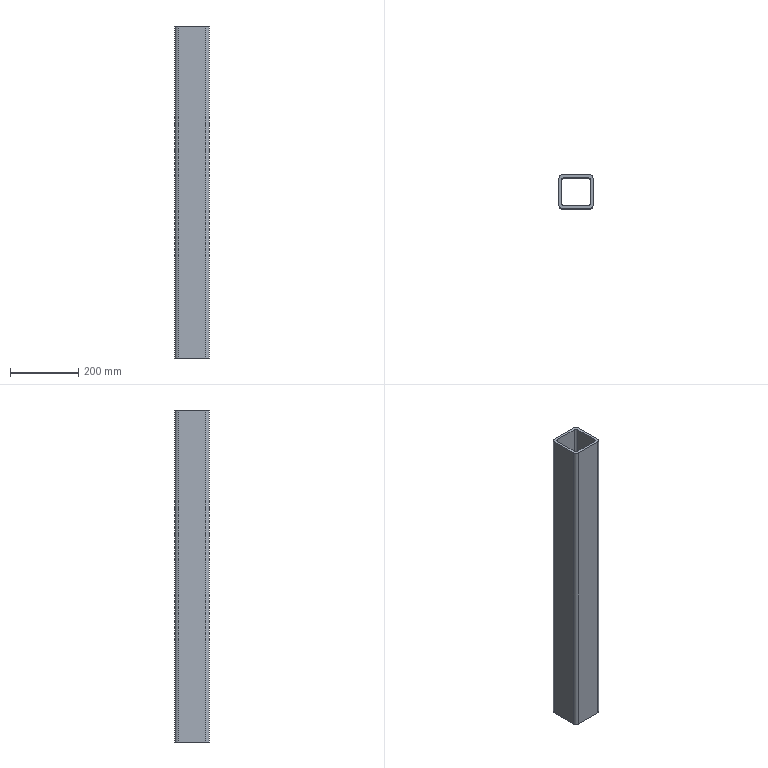Part | SolidWorks | features BaseBody 1 | 1 solid | 18 faces | box 100 x 100 x 976 mm | volume 2843183 mm3 | plane 10 | cylinder 8 | commonest cylinder face diameters 16 x4 20 x4
STEP:
#1=CARTESIAN_POINT('',(90.,-3.65,976.));
#2=VERTEX_POINT('',#1);
#3=CARTESIAN_POINT('',(90.,-3.65,0.));
#4=VERTEX_POINT('',#3);
#5=CARTESIAN_POINT('',(90.,-3.65,976.));
#6=DIRECTION('',(0.,0.,-1.));
#7=VECTOR('',#6,1000.);
#8=LINE('',#5,#7);
#9=EDGE_CURVE('',#2,#4,#8,.T.);
#10=ORIENTED_EDGE('',*,*,#9,.F.);
#11=CARTESIAN_POINT('',(10.,-3.65,976.));
#12=VERTEX_POINT('',#11);
#13=CARTESIAN_POINT('',(10.,-3.65,976.));
#14=DIRECTION('',(1.,0.,0.));
#15=VECTOR('',#14,1000.);
#16=LINE('',#13,#15);
#17=EDGE_CURVE('',#12,#2,#16,.T.);
#18=ORIENTED_EDGE('',*,*,#17,.F.);
#19=CARTESIAN_POINT('',(10.,-3.65,0.));
#20=VERTEX_POINT('',#19);
#21=CARTESIAN_POINT('',(10.,-3.65,976.));
#22=DIRECTION('',(0.,0.,1.));
#23=VECTOR('',#22,1000.);
#24=LINE('',#21,#23);
#25=EDGE_CURVE('',#20,#12,#24,.T.);
#26=ORIENTED_EDGE('',*,*,#25,.F.);
#27=CARTESIAN_POINT('',(10.,-3.65,0.));
#28=DIRECTION('',(-1.,0.,0.));
#29=VECTOR('',#28,1000.);
#30=LINE('',#27,#29);
#31=EDGE_CURVE('',#4,#20,#30,.T.);
#32=ORIENTED_EDGE('',*,*,#31,.F.);
#33=EDGE_LOOP('',(#10,#18,#26,#32));
#34=FACE_OUTER_BOUND('',#33,.T.);
#35=CARTESIAN_POINT('',(10.,-3.65,976.));
#36=DIRECTION('',(0.,1.,0.));
#37=DIRECTION('',(-1.,0.,0.));
#38=AXIS2_PLACEMENT_3D('',#35,#36,#37);
#39=PLANE('',#38);
#40=ADVANCED_FACE('',(#34),#39,.F.);
#41=CARTESIAN_POINT('',(84.,4.35,0.));
#42=VERTEX_POINT('',#41);
#43=CARTESIAN_POINT('',(16.,4.35,0.));
#44=VERTEX_POINT('',#43);
#45=CARTESIAN_POINT('',(10.,4.35,0.));
#46=DIRECTION('',(-1.,0.,0.));
#47=VECTOR('',#46,1000.);
#48=LINE('',#45,#47);
#49=EDGE_CURVE('',#42,#44,#48,.T.);
#50=ORIENTED_EDGE('',*,*,#49,.F.);
#51=CARTESIAN_POINT('',(92.,12.35,0.));
#52=VERTEX_POINT('',#51);
#53=CARTESIAN_POINT('',(84.,12.35,0.));
#54=DIRECTION('',(0.,0.,-1.));
#55=DIRECTION('',(-1.,0.,0.));
#56=AXIS2_PLACEMENT_3D('',#53,#54,#55);
#57=CIRCLE('',#56,8.);
#58=EDGE_CURVE('',#52,#42,#57,.T.);
#59=ORIENTED_EDGE('',*,*,#58,.F.);
#60=CARTESIAN_POINT('',(92.,80.35,0.));
#61=VERTEX_POINT('',#60);
#62=CARTESIAN_POINT('',(92.,6.35,0.));
#63=DIRECTION('',(0.,-1.,0.));
#64=VECTOR('',#63,1000.);
#65=LINE('',#62,#64);
#66=EDGE_CURVE('',#61,#52,#65,.T.);
#67=ORIENTED_EDGE('',*,*,#66,.F.);
#68=CARTESIAN_POINT('',(84.,88.35,0.));
#69=VERTEX_POINT('',#68);
#70=CARTESIAN_POINT('',(84.,80.35,0.));
#71=DIRECTION('',(0.,0.,-1.));
#72=DIRECTION('',(-1.,0.,0.));
#73=AXIS2_PLACEMENT_3D('',#70,#71,#72);
#74=CIRCLE('',#73,8.);
#75=EDGE_CURVE('',#69,#61,#74,.T.);
#76=ORIENTED_EDGE('',*,*,#75,.F.);
#77=CARTESIAN_POINT('',(16.,88.35,0.));
#78=VERTEX_POINT('',#77);
#79=CARTESIAN_POINT('',(10.,88.35,0.));
#80=DIRECTION('',(1.,0.,0.));
#81=VECTOR('',#80,1000.);
#82=LINE('',#79,#81);
#83=EDGE_CURVE('',#78,#69,#82,.T.);
#84=ORIENTED_EDGE('',*,*,#83,.F.);
#85=CARTESIAN_POINT('',(8.,80.35,0.));
#86=VERTEX_POINT('',#85);
#87=CARTESIAN_POINT('',(16.,80.35,0.));
#88=DIRECTION('',(0.,0.,-1.));
#89=DIRECTION('',(-1.,0.,0.));
#90=AXIS2_PLACEMENT_3D('',#87,#88,#89);
#91=CIRCLE('',#90,8.);
#92=EDGE_CURVE('',#86,#78,#91,.T.);
#93=ORIENTED_EDGE('',*,*,#92,.F.);
#94=CARTESIAN_POINT('',(8.,12.35,0.));
#95=VERTEX_POINT('',#94);
#96=CARTESIAN_POINT('',(8.,6.35,0.));
#97=DIRECTION('',(0.,1.,0.));
#98=VECTOR('',#97,1000.);
#99=LINE('',#96,#98);
#100=EDGE_CURVE('',#95,#86,#99,.T.);
#101=ORIENTED_EDGE('',*,*,#100,.F.);
#102=CARTESIAN_POINT('',(16.,12.35,0.));
#103=DIRECTION('',(0.,0.,-1.));
#104=DIRECTION('',(-1.,0.,0.));
#105=AXIS2_PLACEMENT_3D('',#102,#103,#104);
#106=CIRCLE('',#105,8.);
#107=EDGE_CURVE('',#44,#95,#106,.T.);
#108=ORIENTED_EDGE('',*,*,#107,.F.);
#109=EDGE_LOOP('',(#50,#59,#67,#76,#84,#93,#101,#108));
#110=FACE_BOUND('',#109,.T.);
#111=CARTESIAN_POINT('',(0.,86.35,0.));
#112=VERTEX_POINT('',#111);
#113=CARTESIAN_POINT('',(0.,6.35,0.));
#114=VERTEX_POINT('',#113);
#115=CARTESIAN_POINT('',(0.,6.35,0.));
#116=DIRECTION('',(0.,-1.,0.));
#117=VECTOR('',#116,1000.);
#118=LINE('',#115,#117);
#119=EDGE_CURVE('',#112,#114,#118,.T.);
#120=ORIENTED_EDGE('',*,*,#119,.F.);
#121=CARTESIAN_POINT('',(10.,96.35,0.));
#122=VERTEX_POINT('',#121);
#123=CARTESIAN_POINT('',(10.,86.35,0.));
#124=DIRECTION('',(0.,0.,1.));
#125=DIRECTION('',(-1.,0.,0.));
#126=AXIS2_PLACEMENT_3D('',#123,#124,#125);
#127=CIRCLE('',#126,10.);
#128=EDGE_CURVE('',#122,#112,#127,.T.);
#129=ORIENTED_EDGE('',*,*,#128,.F.);
#130=CARTESIAN_POINT('',(90.,96.35,0.));
#131=VERTEX_POINT('',#130);
#132=CARTESIAN_POINT('',(10.,96.35,0.));
#133=DIRECTION('',(-1.,0.,0.));
#134=VECTOR('',#133,1000.);
#135=LINE('',#132,#134);
#136=EDGE_CURVE('',#131,#122,#135,.T.);
#137=ORIENTED_EDGE('',*,*,#136,.F.);
#138=CARTESIAN_POINT('',(100.,86.35,0.));
#139=VERTEX_POINT('',#138);
#140=CARTESIAN_POINT('',(90.,86.35,0.));
#141=DIRECTION('',(0.,0.,1.));
#142=DIRECTION('',(-1.,0.,0.));
#143=AXIS2_PLACEMENT_3D('',#140,#141,#142);
#144=CIRCLE('',#143,10.);
#145=EDGE_CURVE('',#139,#131,#144,.T.);
#146=ORIENTED_EDGE('',*,*,#145,.F.);
#147=CARTESIAN_POINT('',(100.,6.35,0.));
#148=VERTEX_POINT('',#147);
#149=CARTESIAN_POINT('',(100.,6.35,0.));
#150=DIRECTION('',(0.,1.,0.));
#151=VECTOR('',#150,1000.);
#152=LINE('',#149,#151);
#153=EDGE_CURVE('',#148,#139,#152,.T.);
#154=ORIENTED_EDGE('',*,*,#153,.F.);
#155=CARTESIAN_POINT('',(90.,6.35,0.));
#156=DIRECTION('',(0.,0.,1.));
#157=DIRECTION('',(-1.,0.,0.));
#158=AXIS2_PLACEMENT_3D('',#155,#156,#157);
#159=CIRCLE('',#158,10.);
#160=EDGE_CURVE('',#4,#148,#159,.T.);
#161=ORIENTED_EDGE('',*,*,#160,.F.);
#162=ORIENTED_EDGE('',*,*,#31,.T.);
#163=CARTESIAN_POINT('',(10.,6.35,0.));
#164=DIRECTION('',(0.,0.,1.));
#165=DIRECTION('',(-1.,0.,0.));
#166=AXIS2_PLACEMENT_3D('',#163,#164,#165);
#167=CIRCLE('',#166,10.);
#168=EDGE_CURVE('',#114,#20,#167,.T.);
#169=ORIENTED_EDGE('',*,*,#168,.F.);
#170=EDGE_LOOP('',(#120,#129,#137,#146,#154,#161,#162,#169));
#171=FACE_OUTER_BOUND('',#170,.T.);
#172=CARTESIAN_POINT('',(10.,6.35,0.));
#173=DIRECTION('',(0.,0.,1.));
#174=DIRECTION('',(1.,0.,0.));
#175=AXIS2_PLACEMENT_3D('',#172,#173,#174);
#176=PLANE('',#175);
#177=ADVANCED_FACE('',(#110,#171),#176,.F.);
#178=CARTESIAN_POINT('',(100.,6.35,976.));
#179=VERTEX_POINT('',#178);
#180=CARTESIAN_POINT('',(90.,6.35,976.));
#181=DIRECTION('',(0.,0.,-1.));
#182=DIRECTION('',(-1.,0.,0.));
#183=AXIS2_PLACEMENT_3D('',#180,#181,#182);
#184=CIRCLE('',#183,10.);
#185=EDGE_CURVE('',#179,#2,#184,.T.);
#186=ORIENTED_EDGE('',*,*,#185,.T.);
#187=ORIENTED_EDGE('',*,*,#9,.T.);
#188=ORIENTED_EDGE('',*,*,#160,.T.);
#189=CARTESIAN_POINT('',(100.,6.35,976.));
#190=DIRECTION('',(0.,0.,1.));
#191=VECTOR('',#190,1000.);
#192=LINE('',#189,#191);
#193=EDGE_CURVE('',#148,#179,#192,.T.);
#194=ORIENTED_EDGE('',*,*,#193,.T.);
#195=EDGE_LOOP('',(#186,#187,#188,#194));
#196=FACE_OUTER_BOUND('',#195,.T.);
#197=CARTESIAN_POINT('',(90.,6.35,976.));
#198=DIRECTION('',(0.,0.,-1.));
#199=DIRECTION('',(-1.,0.,0.));
#200=AXIS2_PLACEMENT_3D('',#197,#198,#199);
#201=CYLINDRICAL_SURFACE('',#200,10.);
#202=ADVANCED_FACE('',(#196),#201,.T.);
#203=CARTESIAN_POINT('',(92.,80.35,976.));
#204=VERTEX_POINT('',#203);
#205=CARTESIAN_POINT('',(92.,12.35,976.));
#206=VERTEX_POINT('',#205);
#207=CARTESIAN_POINT('',(92.,6.35,976.));
#208=DIRECTION('',(0.,-1.,0.));
#209=VECTOR('',#208,1000.);
#210=LINE('',#207,#209);
#211=EDGE_CURVE('',#204,#206,#210,.T.);
#212=ORIENTED_EDGE('',*,*,#211,.T.);
#213=CARTESIAN_POINT('',(84.,4.35,976.));
#214=VERTEX_POINT('',#213);
#215=CARTESIAN_POINT('',(84.,12.35,976.));
#216=DIRECTION('',(0.,0.,-1.));
#217=DIRECTION('',(-1.,0.,0.));
#218=AXIS2_PLACEMENT_3D('',#215,#216,#217);
#219=CIRCLE('',#218,8.);
#220=EDGE_CURVE('',#206,#214,#219,.T.);
#221=ORIENTED_EDGE('',*,*,#220,.T.);
#222=CARTESIAN_POINT('',(16.,4.35,976.));
#223=VERTEX_POINT('',#222);
#224=CARTESIAN_POINT('',(10.,4.35,976.));
#225=DIRECTION('',(-1.,0.,0.));
#226=VECTOR('',#225,1000.);
#227=LINE('',#224,#226);
#228=EDGE_CURVE('',#214,#223,#227,.T.);
#229=ORIENTED_EDGE('',*,*,#228,.T.);
#230=CARTESIAN_POINT('',(8.,12.35,976.));
#231=VERTEX_POINT('',#230);
#232=CARTESIAN_POINT('',(16.,12.35,976.));
#233=DIRECTION('',(0.,0.,-1.));
#234=DIRECTION('',(-1.,0.,0.));
#235=AXIS2_PLACEMENT_3D('',#232,#233,#234);
#236=CIRCLE('',#235,8.);
#237=EDGE_CURVE('',#223,#231,#236,.T.);
#238=ORIENTED_EDGE('',*,*,#237,.T.);
#239=CARTESIAN_POINT('',(8.,80.35,976.));
#240=VERTEX_POINT('',#239);
#241=CARTESIAN_POINT('',(8.,6.35,976.));
#242=DIRECTION('',(0.,1.,0.));
#243=VECTOR('',#242,1000.);
#244=LINE('',#241,#243);
#245=EDGE_CURVE('',#231,#240,#244,.T.);
#246=ORIENTED_EDGE('',*,*,#245,.T.);
#247=CARTESIAN_POINT('',(16.,88.35,976.));
#248=VERTEX_POINT('',#247);
#249=CARTESIAN_POINT('',(16.,80.35,976.));
#250=DIRECTION('',(0.,0.,-1.));
#251=DIRECTION('',(-1.,0.,0.));
#252=AXIS2_PLACEMENT_3D('',#249,#250,#251);
#253=CIRCLE('',#252,8.);
#254=EDGE_CURVE('',#240,#248,#253,.T.);
#255=ORIENTED_EDGE('',*,*,#254,.T.);
#256=CARTESIAN_POINT('',(84.,88.35,976.));
#257=VERTEX_POINT('',#256);
#258=CARTESIAN_POINT('',(10.,88.35,976.));
#259=DIRECTION('',(1.,0.,0.));
#260=VECTOR('',#259,1000.);
#261=LINE('',#258,#260);
#262=EDGE_CURVE('',#248,#257,#261,.T.);
#263=ORIENTED_EDGE('',*,*,#262,.T.);
#264=CARTESIAN_POINT('',(84.,80.35,976.));
#265=DIRECTION('',(0.,0.,-1.));
#266=DIRECTION('',(-1.,0.,0.));
#267=AXIS2_PLACEMENT_3D('',#264,#265,#266);
#268=CIRCLE('',#267,8.);
#269=EDGE_CURVE('',#257,#204,#268,.T.);
#270=ORIENTED_EDGE('',*,*,#269,.T.);
#271=EDGE_LOOP('',(#212,#221,#229,#238,#246,#255,#263,#270));
#272=FACE_BOUND('',#271,.T.);
#273=CARTESIAN_POINT('',(10.,96.35,976.));
#274=VERTEX_POINT('',#273);
#275=CARTESIAN_POINT('',(0.,86.35,976.));
#276=VERTEX_POINT('',#275);
#277=CARTESIAN_POINT('',(10.,86.35,976.));
#278=DIRECTION('',(0.,0.,1.));
#279=DIRECTION('',(-1.,0.,0.));
#280=AXIS2_PLACEMENT_3D('',#277,#278,#279);
#281=CIRCLE('',#280,10.);
#282=EDGE_CURVE('',#274,#276,#281,.T.);
#283=ORIENTED_EDGE('',*,*,#282,.T.);
#284=CARTESIAN_POINT('',(0.,6.35,976.));
#285=VERTEX_POINT('',#284);
#286=CARTESIAN_POINT('',(0.,6.35,976.));
#287=DIRECTION('',(0.,-1.,0.));
#288=VECTOR('',#287,1000.);
#289=LINE('',#286,#288);
#290=EDGE_CURVE('',#276,#285,#289,.T.);
#291=ORIENTED_EDGE('',*,*,#290,.T.);
#292=CARTESIAN_POINT('',(10.,6.35,976.));
#293=DIRECTION('',(0.,0.,1.));
#294=DIRECTION('',(-1.,0.,0.));
#295=AXIS2_PLACEMENT_3D('',#292,#293,#294);
#296=CIRCLE('',#295,10.);
#297=EDGE_CURVE('',#285,#12,#296,.T.);
#298=ORIENTED_EDGE('',*,*,#297,.T.);
#299=ORIENTED_EDGE('',*,*,#17,.T.);
#300=ORIENTED_EDGE('',*,*,#185,.F.);
#301=CARTESIAN_POINT('',(100.,86.35,976.));
#302=VERTEX_POINT('',#301);
#303=CARTESIAN_POINT('',(100.,6.35,976.));
#304=DIRECTION('',(0.,1.,0.));
#305=VECTOR('',#304,1000.);
#306=LINE('',#303,#305);
#307=EDGE_CURVE('',#179,#302,#306,.T.);
#308=ORIENTED_EDGE('',*,*,#307,.T.);
#309=CARTESIAN_POINT('',(90.,96.35,976.));
#310=VERTEX_POINT('',#309);
#311=CARTESIAN_POINT('',(90.,86.35,976.));
#312=DIRECTION('',(0.,0.,1.));
#313=DIRECTION('',(-1.,0.,0.));
#314=AXIS2_PLACEMENT_3D('',#311,#312,#313);
#315=CIRCLE('',#314,10.);
#316=EDGE_CURVE('',#302,#310,#315,.T.);
#317=ORIENTED_EDGE('',*,*,#316,.T.);
#318=CARTESIAN_POINT('',(10.,96.35,976.));
#319=DIRECTION('',(-1.,0.,0.));
#320=VECTOR('',#319,1000.);
#321=LINE('',#318,#320);
#322=EDGE_CURVE('',#310,#274,#321,.T.);
#323=ORIENTED_EDGE('',*,*,#322,.T.);
#324=EDGE_LOOP('',(#283,#291,#298,#299,#300,#308,#317,#323));
#325=FACE_OUTER_BOUND('',#324,.T.);
#326=CARTESIAN_POINT('',(10.,6.35,976.));
#327=DIRECTION('',(0.,0.,1.));
#328=DIRECTION('',(1.,0.,0.));
#329=AXIS2_PLACEMENT_3D('',#326,#327,#328);
#330=PLANE('',#329);
#331=ADVANCED_FACE('',(#272,#325),#330,.T.);
#332=ORIENTED_EDGE('',*,*,#297,.F.);
#333=CARTESIAN_POINT('',(0.,6.35,976.));
#334=DIRECTION('',(0.,0.,-1.));
#335=VECTOR('',#334,1000.);
#336=LINE('',#333,#335);
#337=EDGE_CURVE('',#285,#114,#336,.T.);
#338=ORIENTED_EDGE('',*,*,#337,.T.);
#339=ORIENTED_EDGE('',*,*,#168,.T.);
#340=ORIENTED_EDGE('',*,*,#25,.T.);
#341=EDGE_LOOP('',(#332,#338,#339,#340));
#342=FACE_OUTER_BOUND('',#341,.T.);
#343=CARTESIAN_POINT('',(10.,6.35,976.));
#344=DIRECTION('',(0.,0.,-1.));
#345=DIRECTION('',(-1.,0.,0.));
#346=AXIS2_PLACEMENT_3D('',#343,#344,#345);
#347=CYLINDRICAL_SURFACE('',#346,10.);
#348=ADVANCED_FACE('',(#342),#347,.T.);
#349=CARTESIAN_POINT('',(8.,12.35,976.));
#350=DIRECTION('',(0.,0.,-1.));
#351=VECTOR('',#350,1000.);
#352=LINE('',#349,#351);
#353=EDGE_CURVE('',#231,#95,#352,.T.);
#354=ORIENTED_EDGE('',*,*,#353,.F.);
#355=ORIENTED_EDGE('',*,*,#237,.F.);
#356=CARTESIAN_POINT('',(16.,4.35,976.));
#357=DIRECTION('',(0.,0.,1.));
#358=VECTOR('',#357,1000.);
#359=LINE('',#356,#358);
#360=EDGE_CURVE('',#44,#223,#359,.T.);
#361=ORIENTED_EDGE('',*,*,#360,.F.);
#362=ORIENTED_EDGE('',*,*,#107,.T.);
#363=EDGE_LOOP('',(#354,#355,#361,#362));
#364=FACE_OUTER_BOUND('',#363,.T.);
#365=CARTESIAN_POINT('',(16.,12.35,976.));
#366=DIRECTION('',(0.,0.,-1.));
#367=DIRECTION('',(-1.,0.,0.));
#368=AXIS2_PLACEMENT_3D('',#365,#366,#367);
#369=CYLINDRICAL_SURFACE('',#368,8.);
#370=ADVANCED_FACE('',(#364),#369,.F.);
#371=ORIENTED_EDGE('',*,*,#228,.F.);
#372=CARTESIAN_POINT('',(84.,4.35,976.));
#373=DIRECTION('',(0.,0.,-1.));
#374=VECTOR('',#373,1000.);
#375=LINE('',#372,#374);
#376=EDGE_CURVE('',#214,#42,#375,.T.);
#377=ORIENTED_EDGE('',*,*,#376,.T.);
#378=ORIENTED_EDGE('',*,*,#49,.T.);
#379=ORIENTED_EDGE('',*,*,#360,.T.);
#380=EDGE_LOOP('',(#371,#377,#378,#379));
#381=FACE_OUTER_BOUND('',#380,.T.);
#382=CARTESIAN_POINT('',(16.,4.35,976.));
#383=DIRECTION('',(0.,1.,0.));
#384=DIRECTION('',(-1.,0.,0.));
#385=AXIS2_PLACEMENT_3D('',#382,#383,#384);
#386=PLANE('',#385);
#387=ADVANCED_FACE('',(#381),#386,.T.);
#388=ORIENTED_EDGE('',*,*,#376,.F.);
#389=ORIENTED_EDGE('',*,*,#220,.F.);
#390=CARTESIAN_POINT('',(92.,12.35,976.));
#391=DIRECTION('',(0.,0.,1.));
#392=VECTOR('',#391,1000.);
#393=LINE('',#390,#392);
#394=EDGE_CURVE('',#52,#206,#393,.T.);
#395=ORIENTED_EDGE('',*,*,#394,.F.);
#396=ORIENTED_EDGE('',*,*,#58,.T.);
#397=EDGE_LOOP('',(#388,#389,#395,#396));
#398=FACE_OUTER_BOUND('',#397,.T.);
#399=CARTESIAN_POINT('',(84.,12.35,976.));
#400=DIRECTION('',(0.,0.,-1.));
#401=DIRECTION('',(-1.,0.,0.));
#402=AXIS2_PLACEMENT_3D('',#399,#400,#401);
#403=CYLINDRICAL_SURFACE('',#402,8.);
#404=ADVANCED_FACE('',(#398),#403,.F.);
#405=ORIENTED_EDGE('',*,*,#394,.T.);
#406=ORIENTED_EDGE('',*,*,#211,.F.);
#407=CARTESIAN_POINT('',(92.,80.35,976.));
#408=DIRECTION('',(0.,0.,1.));
#409=VECTOR('',#408,1000.);
#410=LINE('',#407,#409);
#411=EDGE_CURVE('',#61,#204,#410,.T.);
#412=ORIENTED_EDGE('',*,*,#411,.F.);
#413=ORIENTED_EDGE('',*,*,#66,.T.);
#414=EDGE_LOOP('',(#405,#406,#412,#413));
#415=FACE_OUTER_BOUND('',#414,.T.);
#416=CARTESIAN_POINT('',(92.,80.35,976.));
#417=DIRECTION('',(1.,0.,0.));
#418=DIRECTION('',(0.,1.,0.));
#419=AXIS2_PLACEMENT_3D('',#416,#417,#418);
#420=PLANE('',#419);
#421=ADVANCED_FACE('',(#415),#420,.F.);
#422=ORIENTED_EDGE('',*,*,#411,.T.);
#423=ORIENTED_EDGE('',*,*,#269,.F.);
#424=CARTESIAN_POINT('',(84.,88.35,976.));
#425=DIRECTION('',(0.,0.,1.));
#426=VECTOR('',#425,1000.);
#427=LINE('',#424,#426);
#428=EDGE_CURVE('',#69,#257,#427,.T.);
#429=ORIENTED_EDGE('',*,*,#428,.F.);
#430=ORIENTED_EDGE('',*,*,#75,.T.);
#431=EDGE_LOOP('',(#422,#423,#429,#430));
#432=FACE_OUTER_BOUND('',#431,.T.);
#433=CARTESIAN_POINT('',(84.,80.35,976.));
#434=DIRECTION('',(0.,0.,-1.));
#435=DIRECTION('',(-1.,0.,0.));
#436=AXIS2_PLACEMENT_3D('',#433,#434,#435);
#437=CYLINDRICAL_SURFACE('',#436,8.);
#438=ADVANCED_FACE('',(#432),#437,.F.);
#439=ORIENTED_EDGE('',*,*,#262,.F.);
#440=CARTESIAN_POINT('',(16.,88.35,976.));
#441=DIRECTION('',(0.,0.,-1.));
#442=VECTOR('',#441,1000.);
#443=LINE('',#440,#442);
#444=EDGE_CURVE('',#248,#78,#443,.T.);
#445=ORIENTED_EDGE('',*,*,#444,.T.);
#446=ORIENTED_EDGE('',*,*,#83,.T.);
#447=ORIENTED_EDGE('',*,*,#428,.T.);
#448=EDGE_LOOP('',(#439,#445,#446,#447));
#449=FACE_OUTER_BOUND('',#448,.T.);
#450=CARTESIAN_POINT('',(84.,88.35,976.));
#451=DIRECTION('',(0.,-1.,0.));
#452=DIRECTION('',(1.,0.,0.));
#453=AXIS2_PLACEMENT_3D('',#450,#451,#452);
#454=PLANE('',#453);
#455=ADVANCED_FACE('',(#449),#454,.T.);
#456=ORIENTED_EDGE('',*,*,#444,.F.);
#457=ORIENTED_EDGE('',*,*,#254,.F.);
#458=CARTESIAN_POINT('',(8.,80.35,976.));
#459=DIRECTION('',(0.,0.,1.));
#460=VECTOR('',#459,1000.);
#461=LINE('',#458,#460);
#462=EDGE_CURVE('',#86,#240,#461,.T.);
#463=ORIENTED_EDGE('',*,*,#462,.F.);
#464=ORIENTED_EDGE('',*,*,#92,.T.);
#465=EDGE_LOOP('',(#456,#457,#463,#464));
#466=FACE_OUTER_BOUND('',#465,.T.);
#467=CARTESIAN_POINT('',(16.,80.35,976.));
#468=DIRECTION('',(0.,0.,-1.));
#469=DIRECTION('',(-1.,0.,0.));
#470=AXIS2_PLACEMENT_3D('',#467,#468,#469);
#471=CYLINDRICAL_SURFACE('',#470,8.);
#472=ADVANCED_FACE('',(#466),#471,.F.);
#473=ORIENTED_EDGE('',*,*,#462,.T.);
#474=ORIENTED_EDGE('',*,*,#245,.F.);
#475=ORIENTED_EDGE('',*,*,#353,.T.);
#476=ORIENTED_EDGE('',*,*,#100,.T.);
#477=EDGE_LOOP('',(#473,#474,#475,#476));
#478=FACE_OUTER_BOUND('',#477,.T.);
#479=CARTESIAN_POINT('',(8.,12.35,976.));
#480=DIRECTION('',(-1.,0.,0.));
#481=DIRECTION('',(0.,-1.,0.));
#482=AXIS2_PLACEMENT_3D('',#479,#480,#481);
#483=PLANE('',#482);
#484=ADVANCED_FACE('',(#478),#483,.F.);
#485=ORIENTED_EDGE('',*,*,#290,.F.);
#486=CARTESIAN_POINT('',(0.,86.35,976.));
#487=DIRECTION('',(0.,0.,-1.));
#488=VECTOR('',#487,1000.);
#489=LINE('',#486,#488);
#490=EDGE_CURVE('',#276,#112,#489,.T.);
#491=ORIENTED_EDGE('',*,*,#490,.T.);
#492=ORIENTED_EDGE('',*,*,#119,.T.);
#493=ORIENTED_EDGE('',*,*,#337,.F.);
#494=EDGE_LOOP('',(#485,#491,#492,#493));
#495=FACE_OUTER_BOUND('',#494,.T.);
#496=CARTESIAN_POINT('',(0.,6.35,976.));
#497=DIRECTION('',(-1.,0.,0.));
#498=DIRECTION('',(0.,-1.,0.));
#499=AXIS2_PLACEMENT_3D('',#496,#497,#498);
#500=PLANE('',#499);
#501=ADVANCED_FACE('',(#495),#500,.T.);
#502=ORIENTED_EDGE('',*,*,#282,.F.);
#503=CARTESIAN_POINT('',(10.,96.35,976.));
#504=DIRECTION('',(0.,0.,-1.));
#505=VECTOR('',#504,1000.);
#506=LINE('',#503,#505);
#507=EDGE_CURVE('',#274,#122,#506,.T.);
#508=ORIENTED_EDGE('',*,*,#507,.T.);
#509=ORIENTED_EDGE('',*,*,#128,.T.);
#510=ORIENTED_EDGE('',*,*,#490,.F.);
#511=EDGE_LOOP('',(#502,#508,#509,#510));
#512=FACE_OUTER_BOUND('',#511,.T.);
#513=CARTESIAN_POINT('',(10.,86.35,976.));
#514=DIRECTION('',(0.,0.,-1.));
#515=DIRECTION('',(-1.,0.,0.));
#516=AXIS2_PLACEMENT_3D('',#513,#514,#515);
#517=CYLINDRICAL_SURFACE('',#516,10.);
#518=ADVANCED_FACE('',(#512),#517,.T.);
#519=ORIENTED_EDGE('',*,*,#507,.F.);
#520=ORIENTED_EDGE('',*,*,#322,.F.);
#521=CARTESIAN_POINT('',(90.,96.35,976.));
#522=DIRECTION('',(0.,0.,1.));
#523=VECTOR('',#522,1000.);
#524=LINE('',#521,#523);
#525=EDGE_CURVE('',#131,#310,#524,.T.);
#526=ORIENTED_EDGE('',*,*,#525,.F.);
#527=ORIENTED_EDGE('',*,*,#136,.T.);
#528=EDGE_LOOP('',(#519,#520,#526,#527));
#529=FACE_OUTER_BOUND('',#528,.T.);
#530=CARTESIAN_POINT('',(90.,96.35,976.));
#531=DIRECTION('',(0.,-1.,0.));
#532=DIRECTION('',(1.,0.,0.));
#533=AXIS2_PLACEMENT_3D('',#530,#531,#532);
#534=PLANE('',#533);
#535=ADVANCED_FACE('',(#529),#534,.F.);
#536=ORIENTED_EDGE('',*,*,#316,.F.);
#537=CARTESIAN_POINT('',(100.,86.35,976.));
#538=DIRECTION('',(0.,0.,-1.));
#539=VECTOR('',#538,1000.);
#540=LINE('',#537,#539);
#541=EDGE_CURVE('',#302,#139,#540,.T.);
#542=ORIENTED_EDGE('',*,*,#541,.T.);
#543=ORIENTED_EDGE('',*,*,#145,.T.);
#544=ORIENTED_EDGE('',*,*,#525,.T.);
#545=EDGE_LOOP('',(#536,#542,#543,#544));
#546=FACE_OUTER_BOUND('',#545,.T.);
#547=CARTESIAN_POINT('',(90.,86.35,976.));
#548=DIRECTION('',(0.,0.,-1.));
#549=DIRECTION('',(-1.,0.,0.));
#550=AXIS2_PLACEMENT_3D('',#547,#548,#549);
#551=CYLINDRICAL_SURFACE('',#550,10.);
#552=ADVANCED_FACE('',(#546),#551,.T.);
#553=ORIENTED_EDGE('',*,*,#307,.F.);
#554=ORIENTED_EDGE('',*,*,#193,.F.);
#555=ORIENTED_EDGE('',*,*,#153,.T.);
#556=ORIENTED_EDGE('',*,*,#541,.F.);
#557=EDGE_LOOP('',(#553,#554,#555,#556));
#558=FACE_OUTER_BOUND('',#557,.T.);
#559=CARTESIAN_POINT('',(100.,86.35,976.));
#560=DIRECTION('',(1.,0.,0.));
#561=DIRECTION('',(0.,0.,-1.));
#562=AXIS2_PLACEMENT_3D('',#559,#560,#561);
#563=PLANE('',#562);
#564=ADVANCED_FACE('',(#558),#563,.T.);
#565=CLOSED_SHELL('',(#40,#177,#202,#331,#348,#370,#387,#404,#421,#438,#455,#472,#484,#501,#518,#535,#552,#564));
#566=MANIFOLD_SOLID_BREP('',#565);
#567=CARTESIAN_POINT('',(0.,0.,0.));
#568=DIRECTION('',(0.,0.,1.));
#569=DIRECTION('',(1.,0.,0.));
#570=AXIS2_PLACEMENT_3D('',#567,#568,#569);
#571=(LENGTH_UNIT()NAMED_UNIT(*)SI_UNIT(.MILLI.,.METRE.));
#572=UNCERTAINTY_MEASURE_WITH_UNIT(LENGTH_MEASURE(0.00001),#571,'','');
#573=(NAMED_UNIT(*)PLANE_ANGLE_UNIT()SI_UNIT($,.RADIAN.));
#574=(NAMED_UNIT(*)SI_UNIT($,.STERADIAN.)SOLID_ANGLE_UNIT());
#575=(GEOMETRIC_REPRESENTATION_CONTEXT(3)GLOBAL_UNCERTAINTY_ASSIGNED_CONTEXT((#572))GLOBAL_UNIT_ASSIGNED_CONTEXT((#571,#573,#574))REPRESENTATION_CONTEXT('',''));
#576=ADVANCED_BREP_SHAPE_REPRESENTATION('',(#566,#570),#575);